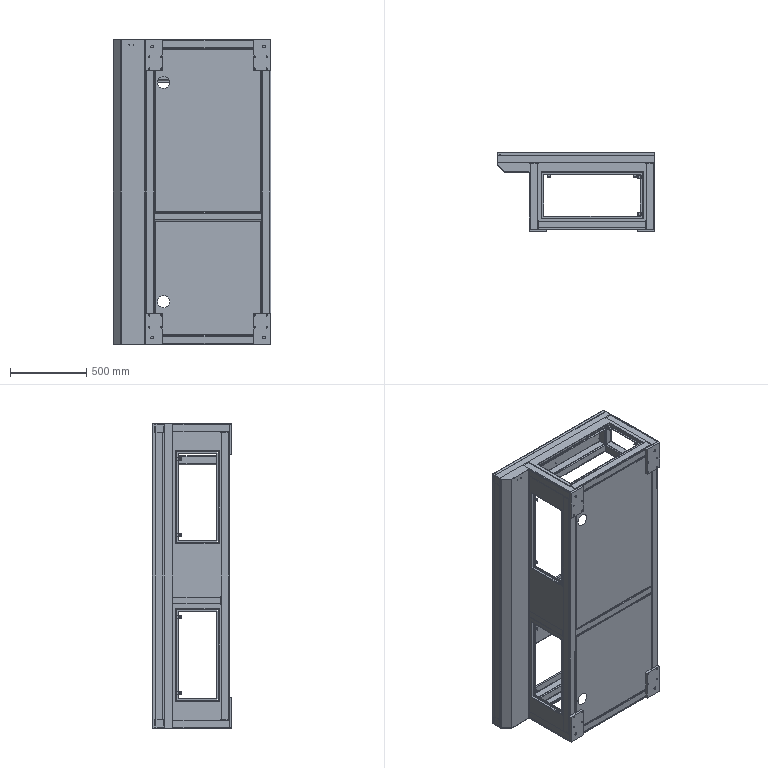Part | NX | features BREP 28 | 28 solids | 1253 faces | box 1035 x 520.5 x 2000 mm | volume 25533043 mm3 | plane 617 | cylinder 513 | spline 84 | cone 39 | commonest cylinder face diameters 7 x79 8 x78 6.8 x77 16 x76 4 x57 8.5 x40